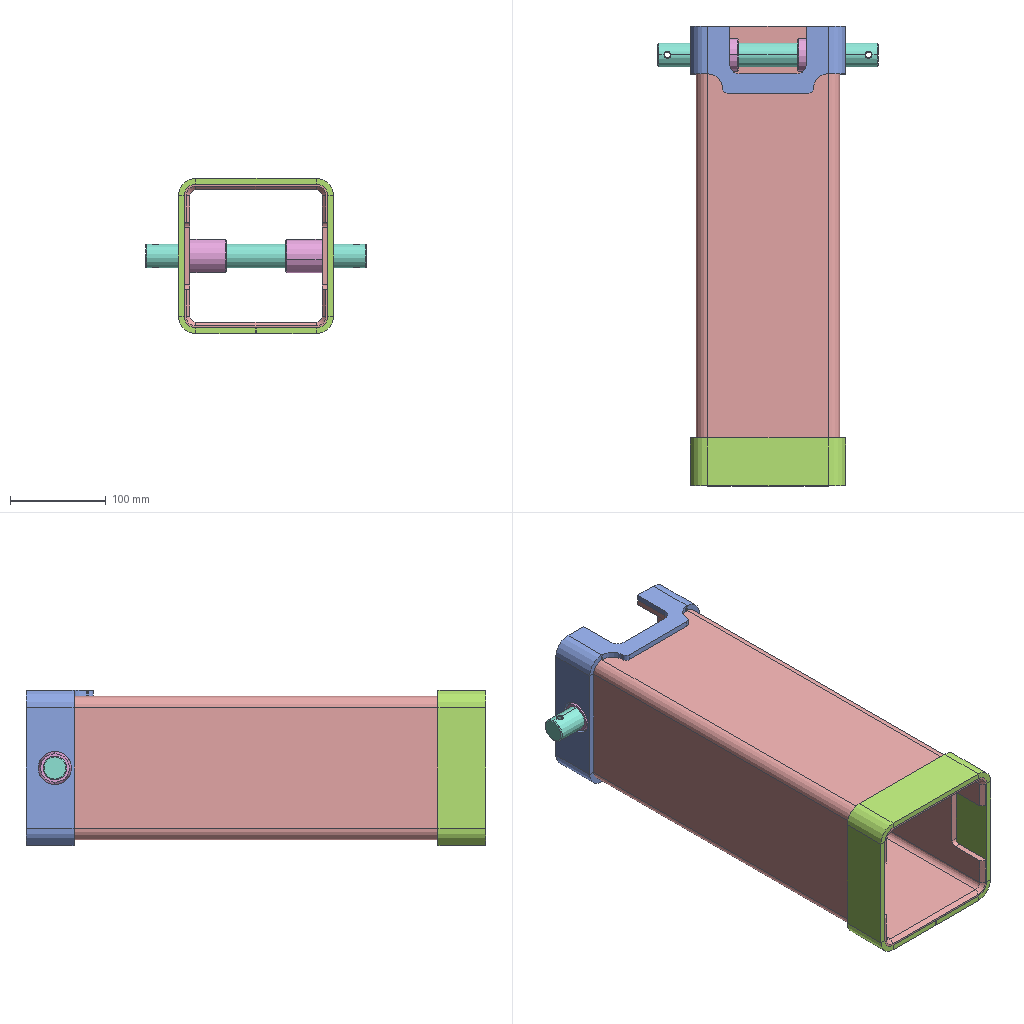Assembly | SolidWorks | 5 different items | 6 placed | box 230 x 480 x 162 mm
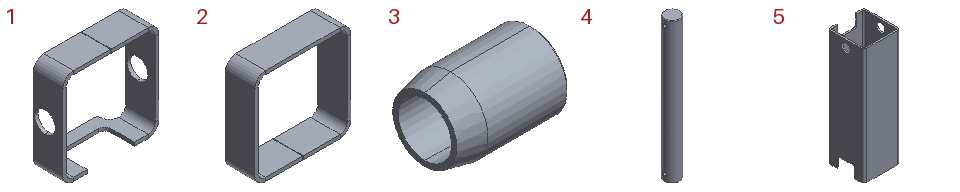Parts list (item | quantity | size | volume | features):
1 | x1 | 162 x 70 x 162 mm | 155802 mm3 | features ICE 2, Fillet 1, FlatPattern 1, SMBaseFlange 1, SheetMetal 1
2 | x1 | 162 x 50 x 162 mm | 179174 mm3 | features FlatPattern 1, SMBaseFlange 1, SheetMetal 1
3 | x2 | 50 x 35 x 35 mm | 21897 mm3 | features Chamfer 1, Revolution 1
4 | x1 | 25 x 25 x 230 mm | 111397 mm3 | features Chamfer 2, Extrusion 1, ICE 1
5 | x1 | 150 x 150 x 480 mm | 1538140 mm3 | features ICE 2, Attribute 1, Chamfer 1, Extrusion 1
Mates (type | each side: item.copy, entity, surface, feature):
Concentric | 5.1 face cylinder Cut-Extrude2 | 1.1 face cylinder Cut-Extrude1
Coincident | 5.1 face plane Boss-Extrude1 | 1.1 face plane Base-Flange1 | 2 times
Coincident | 5.1 face plane Boss-Extrude1 | 2.1 face plane Base-Flange1 | 3 times
Concentric | 5.1 face cylinder Cut-Extrude2 | 3.1 face cylinder Revolve1
Coincident | 1.1 face plane Base-Flange1 | 3.1 face plane Revolve1
Concentric | 5.1 face cylinder Cut-Extrude2 | 3.2 face cylinder Revolve1
Coincident | 1.1 face plane Base-Flange1 | 3.2 face plane Revolve1
Concentric | 3.2 face cylinder Revolve1 | 4.1 face cylinder Boss-Extrude1
DistanceDim | 1.1 face plane Base-Flange1 | 4.1 face plane Boss-Extrude1
Parallel | 1.1 face plane Base-Flange1 | 4.1 plane
Parallel | 3.1 plane | assembly plane | 2 times